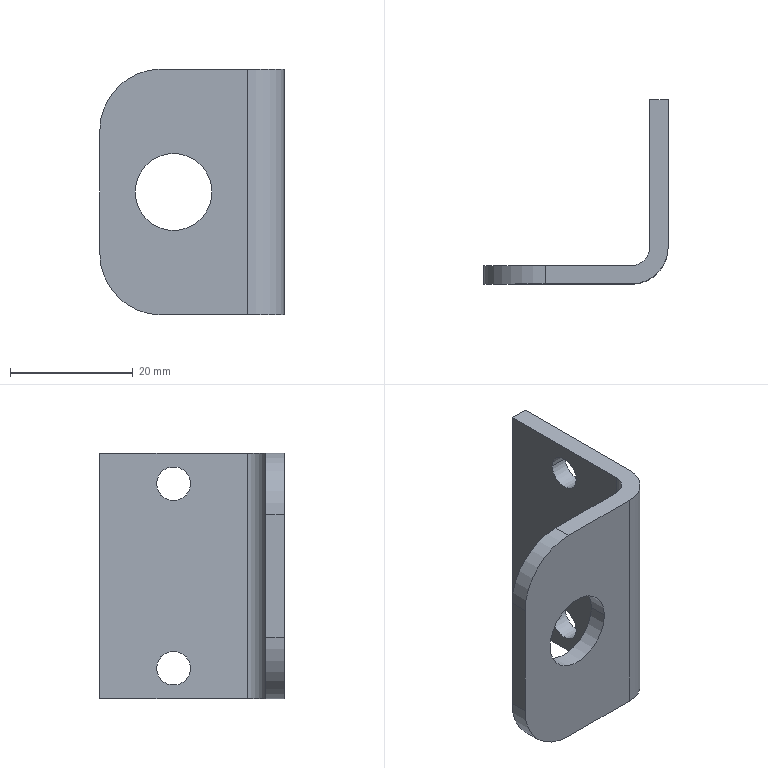Part | STEP file | X77-04002 | 1 solid | 18 faces | box 30 x 30 x 40 mm | volume 5969 mm3 | cylinder 10 | plane 8 | commonest cylinder face diameters 5.5 x4 12.5 x2 20 x2 6 x1 12 x1
STEP:
#1=CARTESIAN_POINT('',(-8.75,-30.,20.));
#2=VERTEX_POINT('',#1);
#3=CARTESIAN_POINT('',(-21.25,-30.,20.));
#4=VERTEX_POINT('',#3);
#5=CARTESIAN_POINT('',(-15.,-30.,20.));
#6=DIRECTION('',(0.,1.,0.));
#7=DIRECTION('',(-1.,0.,0.));
#8=AXIS2_PLACEMENT_3D('',#5,#6,#7);
#9=CIRCLE('',#8,6.25);
#10=EDGE_CURVE('',#2,#4,#9,.T.);
#11=ORIENTED_EDGE('',*,*,#10,.F.);
#12=CARTESIAN_POINT('',(-8.75,-27.,20.));
#13=VERTEX_POINT('',#12);
#14=CARTESIAN_POINT('',(-8.75,-30.,20.));
#15=DIRECTION('',(0.,1.,0.));
#16=VECTOR('',#15,1000.);
#17=LINE('',#14,#16);
#18=EDGE_CURVE('',#2,#13,#17,.T.);
#19=ORIENTED_EDGE('',*,*,#18,.T.);
#20=CARTESIAN_POINT('',(-21.25,-27.,20.));
#21=VERTEX_POINT('',#20);
#22=CARTESIAN_POINT('',(-15.,-27.,20.));
#23=DIRECTION('',(0.,1.,0.));
#24=DIRECTION('',(-1.,0.,0.));
#25=AXIS2_PLACEMENT_3D('',#22,#23,#24);
#26=CIRCLE('',#25,6.25);
#27=EDGE_CURVE('',#13,#21,#26,.T.);
#28=ORIENTED_EDGE('',*,*,#27,.T.);
#29=CARTESIAN_POINT('',(-21.25,-30.,20.));
#30=DIRECTION('',(0.,1.,0.));
#31=VECTOR('',#30,1000.);
#32=LINE('',#29,#31);
#33=EDGE_CURVE('',#4,#21,#32,.T.);
#34=ORIENTED_EDGE('',*,*,#33,.F.);
#35=EDGE_LOOP('',(#11,#19,#28,#34));
#36=FACE_OUTER_BOUND('',#35,.T.);
#37=CARTESIAN_POINT('',(-15.,-30.,20.));
#38=DIRECTION('',(0.,1.,0.));
#39=DIRECTION('',(-1.,0.,0.));
#40=AXIS2_PLACEMENT_3D('',#37,#38,#39);
#41=CYLINDRICAL_SURFACE('',#40,6.25);
#42=ADVANCED_FACE('',(#36),#41,.F.);
#43=CARTESIAN_POINT('',(3.,-9.25,35.));
#44=VERTEX_POINT('',#43);
#45=CARTESIAN_POINT('',(3.,-14.75,35.));
#46=VERTEX_POINT('',#45);
#47=CARTESIAN_POINT('',(3.,-12.,35.));
#48=DIRECTION('',(-1.,0.,0.));
#49=DIRECTION('',(0.,-1.,0.));
#50=AXIS2_PLACEMENT_3D('',#47,#48,#49);
#51=CIRCLE('',#50,2.75);
#52=EDGE_CURVE('',#44,#46,#51,.T.);
#53=ORIENTED_EDGE('',*,*,#52,.F.);
#54=CARTESIAN_POINT('',(0.,-9.25,35.));
#55=VERTEX_POINT('',#54);
#56=CARTESIAN_POINT('',(3.,-9.25,35.));
#57=DIRECTION('',(-1.,0.,0.));
#58=VECTOR('',#57,1000.);
#59=LINE('',#56,#58);
#60=EDGE_CURVE('',#44,#55,#59,.T.);
#61=ORIENTED_EDGE('',*,*,#60,.T.);
#62=CARTESIAN_POINT('',(0.,-14.75,35.));
#63=VERTEX_POINT('',#62);
#64=CARTESIAN_POINT('',(0.,-12.,35.));
#65=DIRECTION('',(-1.,0.,0.));
#66=DIRECTION('',(0.,-1.,0.));
#67=AXIS2_PLACEMENT_3D('',#64,#65,#66);
#68=CIRCLE('',#67,2.75);
#69=EDGE_CURVE('',#55,#63,#68,.T.);
#70=ORIENTED_EDGE('',*,*,#69,.T.);
#71=CARTESIAN_POINT('',(3.,-14.75,35.));
#72=DIRECTION('',(-1.,0.,0.));
#73=VECTOR('',#72,1000.);
#74=LINE('',#71,#73);
#75=EDGE_CURVE('',#46,#63,#74,.T.);
#76=ORIENTED_EDGE('',*,*,#75,.F.);
#77=EDGE_LOOP('',(#53,#61,#70,#76));
#78=FACE_OUTER_BOUND('',#77,.T.);
#79=CARTESIAN_POINT('',(3.,-12.,35.));
#80=DIRECTION('',(-1.,0.,0.));
#81=DIRECTION('',(0.,-1.,0.));
#82=AXIS2_PLACEMENT_3D('',#79,#80,#81);
#83=CYLINDRICAL_SURFACE('',#82,2.75);
#84=ADVANCED_FACE('',(#78),#83,.F.);
#85=CARTESIAN_POINT('',(3.,-9.25,5.));
#86=VERTEX_POINT('',#85);
#87=CARTESIAN_POINT('',(3.,-14.75,5.));
#88=VERTEX_POINT('',#87);
#89=CARTESIAN_POINT('',(3.,-12.,5.));
#90=DIRECTION('',(-1.,0.,0.));
#91=DIRECTION('',(0.,-1.,0.));
#92=AXIS2_PLACEMENT_3D('',#89,#90,#91);
#93=CIRCLE('',#92,2.75);
#94=EDGE_CURVE('',#86,#88,#93,.T.);
#95=ORIENTED_EDGE('',*,*,#94,.F.);
#96=CARTESIAN_POINT('',(0.,-9.25,5.));
#97=VERTEX_POINT('',#96);
#98=CARTESIAN_POINT('',(3.,-9.25,5.));
#99=DIRECTION('',(-1.,0.,0.));
#100=VECTOR('',#99,1000.);
#101=LINE('',#98,#100);
#102=EDGE_CURVE('',#86,#97,#101,.T.);
#103=ORIENTED_EDGE('',*,*,#102,.T.);
#104=CARTESIAN_POINT('',(0.,-14.75,5.));
#105=VERTEX_POINT('',#104);
#106=CARTESIAN_POINT('',(0.,-12.,5.));
#107=DIRECTION('',(-1.,0.,0.));
#108=DIRECTION('',(0.,-1.,0.));
#109=AXIS2_PLACEMENT_3D('',#106,#107,#108);
#110=CIRCLE('',#109,2.75);
#111=EDGE_CURVE('',#97,#105,#110,.T.);
#112=ORIENTED_EDGE('',*,*,#111,.T.);
#113=CARTESIAN_POINT('',(3.,-14.75,5.));
#114=DIRECTION('',(-1.,0.,0.));
#115=VECTOR('',#114,1000.);
#116=LINE('',#113,#115);
#117=EDGE_CURVE('',#88,#105,#116,.T.);
#118=ORIENTED_EDGE('',*,*,#117,.F.);
#119=EDGE_LOOP('',(#95,#103,#112,#118));
#120=FACE_OUTER_BOUND('',#119,.T.);
#121=CARTESIAN_POINT('',(3.,-12.,5.));
#122=DIRECTION('',(-1.,0.,0.));
#123=DIRECTION('',(0.,-1.,0.));
#124=AXIS2_PLACEMENT_3D('',#121,#122,#123);
#125=CYLINDRICAL_SURFACE('',#124,2.75);
#126=ADVANCED_FACE('',(#120),#125,.F.);
#127=CARTESIAN_POINT('',(3.,0.,0.));
#128=VERTEX_POINT('',#127);
#129=CARTESIAN_POINT('',(0.,0.,0.));
#130=VERTEX_POINT('',#129);
#131=CARTESIAN_POINT('',(3.,0.,0.));
#132=DIRECTION('',(-1.,0.,0.));
#133=VECTOR('',#132,1000.);
#134=LINE('',#131,#133);
#135=EDGE_CURVE('',#128,#130,#134,.T.);
#136=ORIENTED_EDGE('',*,*,#135,.T.);
#137=CARTESIAN_POINT('',(0.,0.,40.));
#138=VERTEX_POINT('',#137);
#139=CARTESIAN_POINT('',(0.,0.,40.));
#140=DIRECTION('',(0.,0.,-1.));
#141=VECTOR('',#140,1000.);
#142=LINE('',#139,#141);
#143=EDGE_CURVE('',#138,#130,#142,.T.);
#144=ORIENTED_EDGE('',*,*,#143,.F.);
#145=CARTESIAN_POINT('',(3.,0.,40.));
#146=VERTEX_POINT('',#145);
#147=CARTESIAN_POINT('',(3.,0.,40.));
#148=DIRECTION('',(-1.,0.,0.));
#149=VECTOR('',#148,1000.);
#150=LINE('',#147,#149);
#151=EDGE_CURVE('',#146,#138,#150,.T.);
#152=ORIENTED_EDGE('',*,*,#151,.F.);
#153=CARTESIAN_POINT('',(3.,0.,40.));
#154=DIRECTION('',(0.,0.,-1.));
#155=VECTOR('',#154,1000.);
#156=LINE('',#153,#155);
#157=EDGE_CURVE('',#146,#128,#156,.T.);
#158=ORIENTED_EDGE('',*,*,#157,.T.);
#159=EDGE_LOOP('',(#136,#144,#152,#158));
#160=FACE_OUTER_BOUND('',#159,.T.);
#161=CARTESIAN_POINT('',(3.,0.,40.));
#162=DIRECTION('',(0.,-1.,0.));
#163=DIRECTION('',(1.,0.,0.));
#164=AXIS2_PLACEMENT_3D('',#161,#162,#163);
#165=PLANE('',#164);
#166=ADVANCED_FACE('',(#160),#165,.F.);
#167=CARTESIAN_POINT('',(0.,-12.,35.));
#168=DIRECTION('',(-1.,0.,0.));
#169=DIRECTION('',(0.,-1.,0.));
#170=AXIS2_PLACEMENT_3D('',#167,#168,#169);
#171=CIRCLE('',#170,2.75);
#172=EDGE_CURVE('',#63,#55,#171,.T.);
#173=ORIENTED_EDGE('',*,*,#172,.F.);
#174=ORIENTED_EDGE('',*,*,#69,.F.);
#175=EDGE_LOOP('',(#173,#174));
#176=FACE_BOUND('',#175,.T.);
#177=CARTESIAN_POINT('',(0.,-12.,5.));
#178=DIRECTION('',(-1.,0.,0.));
#179=DIRECTION('',(0.,-1.,0.));
#180=AXIS2_PLACEMENT_3D('',#177,#178,#179);
#181=CIRCLE('',#180,2.75);
#182=EDGE_CURVE('',#105,#97,#181,.T.);
#183=ORIENTED_EDGE('',*,*,#182,.F.);
#184=ORIENTED_EDGE('',*,*,#111,.F.);
#185=EDGE_LOOP('',(#183,#184));
#186=FACE_BOUND('',#185,.T.);
#187=CARTESIAN_POINT('',(0.,-24.,0.));
#188=VERTEX_POINT('',#187);
#189=CARTESIAN_POINT('',(0.,0.,0.));
#190=DIRECTION('',(0.,-1.,0.));
#191=VECTOR('',#190,1000.);
#192=LINE('',#189,#191);
#193=EDGE_CURVE('',#130,#188,#192,.T.);
#194=ORIENTED_EDGE('',*,*,#193,.T.);
#195=CARTESIAN_POINT('',(0.,-24.,40.));
#196=VERTEX_POINT('',#195);
#197=CARTESIAN_POINT('',(0.,-24.,40.));
#198=DIRECTION('',(0.,0.,-1.));
#199=VECTOR('',#198,1000.);
#200=LINE('',#197,#199);
#201=EDGE_CURVE('',#196,#188,#200,.T.);
#202=ORIENTED_EDGE('',*,*,#201,.F.);
#203=CARTESIAN_POINT('',(0.,0.,40.));
#204=DIRECTION('',(0.,-1.,0.));
#205=VECTOR('',#204,1000.);
#206=LINE('',#203,#205);
#207=EDGE_CURVE('',#138,#196,#206,.T.);
#208=ORIENTED_EDGE('',*,*,#207,.F.);
#209=ORIENTED_EDGE('',*,*,#143,.T.);
#210=EDGE_LOOP('',(#194,#202,#208,#209));
#211=FACE_OUTER_BOUND('',#210,.T.);
#212=CARTESIAN_POINT('',(0.,0.,40.));
#213=DIRECTION('',(1.,0.,0.));
#214=DIRECTION('',(0.,1.,0.));
#215=AXIS2_PLACEMENT_3D('',#212,#213,#214);
#216=PLANE('',#215);
#217=ADVANCED_FACE('',(#176,#186,#211),#216,.F.);
#218=CARTESIAN_POINT('',(-3.,-27.,0.));
#219=VERTEX_POINT('',#218);
#220=CARTESIAN_POINT('',(-3.,-24.,0.));
#221=DIRECTION('',(0.,0.,-1.));
#222=DIRECTION('',(1.,0.,0.));
#223=AXIS2_PLACEMENT_3D('',#220,#221,#222);
#224=CIRCLE('',#223,3.);
#225=EDGE_CURVE('',#188,#219,#224,.T.);
#226=ORIENTED_EDGE('',*,*,#225,.T.);
#227=CARTESIAN_POINT('',(-3.,-27.,40.));
#228=VERTEX_POINT('',#227);
#229=CARTESIAN_POINT('',(-3.,-27.,40.));
#230=DIRECTION('',(0.,0.,-1.));
#231=VECTOR('',#230,1000.);
#232=LINE('',#229,#231);
#233=EDGE_CURVE('',#228,#219,#232,.T.);
#234=ORIENTED_EDGE('',*,*,#233,.F.);
#235=CARTESIAN_POINT('',(-3.,-24.,40.));
#236=DIRECTION('',(0.,0.,-1.));
#237=DIRECTION('',(1.,0.,0.));
#238=AXIS2_PLACEMENT_3D('',#235,#236,#237);
#239=CIRCLE('',#238,3.);
#240=EDGE_CURVE('',#196,#228,#239,.T.);
#241=ORIENTED_EDGE('',*,*,#240,.F.);
#242=ORIENTED_EDGE('',*,*,#201,.T.);
#243=EDGE_LOOP('',(#226,#234,#241,#242));
#244=FACE_OUTER_BOUND('',#243,.T.);
#245=CARTESIAN_POINT('',(-3.,-24.,40.));
#246=DIRECTION('',(0.,0.,-1.));
#247=DIRECTION('',(-1.,0.,0.));
#248=AXIS2_PLACEMENT_3D('',#245,#246,#247);
#249=CYLINDRICAL_SURFACE('',#248,3.);
#250=ADVANCED_FACE('',(#244),#249,.F.);
#251=CARTESIAN_POINT('',(-15.,-27.,20.));
#252=DIRECTION('',(0.,1.,0.));
#253=DIRECTION('',(-1.,0.,0.));
#254=AXIS2_PLACEMENT_3D('',#251,#252,#253);
#255=CIRCLE('',#254,6.25);
#256=EDGE_CURVE('',#21,#13,#255,.T.);
#257=ORIENTED_EDGE('',*,*,#256,.F.);
#258=ORIENTED_EDGE('',*,*,#27,.F.);
#259=EDGE_LOOP('',(#257,#258));
#260=FACE_BOUND('',#259,.T.);
#261=CARTESIAN_POINT('',(-27.,-27.,30.));
#262=VERTEX_POINT('',#261);
#263=CARTESIAN_POINT('',(-27.,-27.,10.));
#264=VERTEX_POINT('',#263);
#265=CARTESIAN_POINT('',(-27.,-27.,40.));
#266=DIRECTION('',(0.,0.,-1.));
#267=VECTOR('',#266,1000.);
#268=LINE('',#265,#267);
#269=EDGE_CURVE('',#262,#264,#268,.T.);
#270=ORIENTED_EDGE('',*,*,#269,.F.);
#271=CARTESIAN_POINT('',(-17.,-27.,40.));
#272=VERTEX_POINT('',#271);
#273=CARTESIAN_POINT('',(-17.,-27.,30.));
#274=DIRECTION('',(0.,1.,0.));
#275=DIRECTION('',(1.,0.,0.));
#276=AXIS2_PLACEMENT_3D('',#273,#274,#275);
#277=CIRCLE('',#276,10.);
#278=EDGE_CURVE('',#262,#272,#277,.T.);
#279=ORIENTED_EDGE('',*,*,#278,.T.);
#280=CARTESIAN_POINT('',(-3.,-27.,40.));
#281=DIRECTION('',(-1.,0.,0.));
#282=VECTOR('',#281,1000.);
#283=LINE('',#280,#282);
#284=EDGE_CURVE('',#228,#272,#283,.T.);
#285=ORIENTED_EDGE('',*,*,#284,.F.);
#286=ORIENTED_EDGE('',*,*,#233,.T.);
#287=CARTESIAN_POINT('',(-17.,-27.,0.));
#288=VERTEX_POINT('',#287);
#289=CARTESIAN_POINT('',(-3.,-27.,0.));
#290=DIRECTION('',(-1.,0.,0.));
#291=VECTOR('',#290,1000.);
#292=LINE('',#289,#291);
#293=EDGE_CURVE('',#219,#288,#292,.T.);
#294=ORIENTED_EDGE('',*,*,#293,.T.);
#295=CARTESIAN_POINT('',(-17.,-27.,10.));
#296=DIRECTION('',(0.,1.,0.));
#297=DIRECTION('',(1.,0.,0.));
#298=AXIS2_PLACEMENT_3D('',#295,#296,#297);
#299=CIRCLE('',#298,10.);
#300=EDGE_CURVE('',#288,#264,#299,.T.);
#301=ORIENTED_EDGE('',*,*,#300,.T.);
#302=EDGE_LOOP('',(#270,#279,#285,#286,#294,#301));
#303=FACE_OUTER_BOUND('',#302,.T.);
#304=CARTESIAN_POINT('',(-3.,-27.,40.));
#305=DIRECTION('',(0.,-1.,0.));
#306=DIRECTION('',(1.,0.,0.));
#307=AXIS2_PLACEMENT_3D('',#304,#305,#306);
#308=PLANE('',#307);
#309=ADVANCED_FACE('',(#260,#303),#308,.F.);
#310=CARTESIAN_POINT('',(-27.,-30.,30.));
#311=VERTEX_POINT('',#310);
#312=CARTESIAN_POINT('',(-27.,-30.,10.));
#313=VERTEX_POINT('',#312);
#314=CARTESIAN_POINT('',(-27.,-30.,40.));
#315=DIRECTION('',(0.,0.,-1.));
#316=VECTOR('',#315,1000.);
#317=LINE('',#314,#316);
#318=EDGE_CURVE('',#311,#313,#317,.T.);
#319=ORIENTED_EDGE('',*,*,#318,.F.);
#320=CARTESIAN_POINT('',(-27.,-27.,30.));
#321=DIRECTION('',(0.,1.,0.));
#322=VECTOR('',#321,1000.);
#323=LINE('',#320,#322);
#324=EDGE_CURVE('',#311,#262,#323,.T.);
#325=ORIENTED_EDGE('',*,*,#324,.T.);
#326=ORIENTED_EDGE('',*,*,#269,.T.);
#327=CARTESIAN_POINT('',(-27.,-27.,10.));
#328=DIRECTION('',(0.,-1.,0.));
#329=VECTOR('',#328,1000.);
#330=LINE('',#327,#329);
#331=EDGE_CURVE('',#264,#313,#330,.T.);
#332=ORIENTED_EDGE('',*,*,#331,.T.);
#333=EDGE_LOOP('',(#319,#325,#326,#332));
#334=FACE_OUTER_BOUND('',#333,.T.);
#335=CARTESIAN_POINT('',(-27.,-27.,40.));
#336=DIRECTION('',(1.,0.,0.));
#337=DIRECTION('',(0.,1.,0.));
#338=AXIS2_PLACEMENT_3D('',#335,#336,#337);
#339=PLANE('',#338);
#340=ADVANCED_FACE('',(#334),#339,.F.);
#341=CARTESIAN_POINT('',(-15.,-30.,20.));
#342=DIRECTION('',(0.,1.,0.));
#343=DIRECTION('',(-1.,0.,0.));
#344=AXIS2_PLACEMENT_3D('',#341,#342,#343);
#345=CIRCLE('',#344,6.25);
#346=EDGE_CURVE('',#4,#2,#345,.T.);
#347=ORIENTED_EDGE('',*,*,#346,.T.);
#348=ORIENTED_EDGE('',*,*,#10,.T.);
#349=EDGE_LOOP('',(#347,#348));
#350=FACE_BOUND('',#349,.T.);
#351=CARTESIAN_POINT('',(-17.,-30.,40.));
#352=VERTEX_POINT('',#351);
#353=CARTESIAN_POINT('',(-3.,-30.,40.));
#354=VERTEX_POINT('',#353);
#355=CARTESIAN_POINT('',(-27.,-30.,40.));
#356=DIRECTION('',(1.,0.,0.));
#357=VECTOR('',#356,1000.);
#358=LINE('',#355,#357);
#359=EDGE_CURVE('',#352,#354,#358,.T.);
#360=ORIENTED_EDGE('',*,*,#359,.F.);
#361=CARTESIAN_POINT('',(-17.,-30.,30.));
#362=DIRECTION('',(0.,-1.,0.));
#363=DIRECTION('',(0.,0.,1.));
#364=AXIS2_PLACEMENT_3D('',#361,#362,#363);
#365=CIRCLE('',#364,10.);
#366=EDGE_CURVE('',#352,#311,#365,.T.);
#367=ORIENTED_EDGE('',*,*,#366,.T.);
#368=ORIENTED_EDGE('',*,*,#318,.T.);
#369=CARTESIAN_POINT('',(-17.,-30.,0.));
#370=VERTEX_POINT('',#369);
#371=CARTESIAN_POINT('',(-17.,-30.,10.));
#372=DIRECTION('',(0.,-1.,0.));
#373=DIRECTION('',(0.,0.,1.));
#374=AXIS2_PLACEMENT_3D('',#371,#372,#373);
#375=CIRCLE('',#374,10.);
#376=EDGE_CURVE('',#313,#370,#375,.T.);
#377=ORIENTED_EDGE('',*,*,#376,.T.);
#378=CARTESIAN_POINT('',(-3.,-30.,0.));
#379=VERTEX_POINT('',#378);
#380=CARTESIAN_POINT('',(-27.,-30.,0.));
#381=DIRECTION('',(1.,0.,0.));
#382=VECTOR('',#381,1000.);
#383=LINE('',#380,#382);
#384=EDGE_CURVE('',#370,#379,#383,.T.);
#385=ORIENTED_EDGE('',*,*,#384,.T.);
#386=CARTESIAN_POINT('',(-3.,-30.,40.));
#387=DIRECTION('',(0.,0.,-1.));
#388=VECTOR('',#387,1000.);
#389=LINE('',#386,#388);
#390=EDGE_CURVE('',#354,#379,#389,.T.);
#391=ORIENTED_EDGE('',*,*,#390,.F.);
#392=EDGE_LOOP('',(#360,#367,#368,#377,#385,#391));
#393=FACE_OUTER_BOUND('',#392,.T.);
#394=CARTESIAN_POINT('',(-27.,-30.,40.));
#395=DIRECTION('',(0.,1.,0.));
#396=DIRECTION('',(0.,0.,1.));
#397=AXIS2_PLACEMENT_3D('',#394,#395,#396);
#398=PLANE('',#397);
#399=ADVANCED_FACE('',(#350,#393),#398,.F.);
#400=CARTESIAN_POINT('',(3.,-24.,0.));
#401=VERTEX_POINT('',#400);
#402=CARTESIAN_POINT('',(-3.,-24.,0.));
#403=DIRECTION('',(0.,0.,1.));
#404=DIRECTION('',(1.,0.,0.));
#405=AXIS2_PLACEMENT_3D('',#402,#403,#404);
#406=CIRCLE('',#405,6.);
#407=EDGE_CURVE('',#379,#401,#406,.T.);
#408=ORIENTED_EDGE('',*,*,#407,.T.);
#409=CARTESIAN_POINT('',(3.,-24.,40.));
#410=VERTEX_POINT('',#409);
#411=CARTESIAN_POINT('',(3.,-24.,40.));
#412=DIRECTION('',(0.,0.,-1.));
#413=VECTOR('',#412,1000.);
#414=LINE('',#411,#413);
#415=EDGE_CURVE('',#410,#401,#414,.T.);
#416=ORIENTED_EDGE('',*,*,#415,.F.);
#417=CARTESIAN_POINT('',(-3.,-24.,40.));
#418=DIRECTION('',(0.,0.,1.));
#419=DIRECTION('',(1.,0.,0.));
#420=AXIS2_PLACEMENT_3D('',#417,#418,#419);
#421=CIRCLE('',#420,6.);
#422=EDGE_CURVE('',#354,#410,#421,.T.);
#423=ORIENTED_EDGE('',*,*,#422,.F.);
#424=ORIENTED_EDGE('',*,*,#390,.T.);
#425=EDGE_LOOP('',(#408,#416,#423,#424));
#426=FACE_OUTER_BOUND('',#425,.T.);
#427=CARTESIAN_POINT('',(-3.,-24.,40.));
#428=DIRECTION('',(0.,0.,-1.));
#429=DIRECTION('',(-1.,0.,0.));
#430=AXIS2_PLACEMENT_3D('',#427,#428,#429);
#431=CYLINDRICAL_SURFACE('',#430,6.);
#432=ADVANCED_FACE('',(#426),#431,.T.);
#433=CARTESIAN_POINT('',(3.,-12.,35.));
#434=DIRECTION('',(-1.,0.,0.));
#435=DIRECTION('',(0.,-1.,0.));
#436=AXIS2_PLACEMENT_3D('',#433,#434,#435);
#437=CIRCLE('',#436,2.75);
#438=EDGE_CURVE('',#46,#44,#437,.T.);
#439=ORIENTED_EDGE('',*,*,#438,.T.);
#440=ORIENTED_EDGE('',*,*,#52,.T.);
#441=EDGE_LOOP('',(#439,#440));
#442=FACE_BOUND('',#441,.T.);
#443=CARTESIAN_POINT('',(3.,-12.,5.));
#444=DIRECTION('',(-1.,0.,0.));
#445=DIRECTION('',(0.,-1.,0.));
#446=AXIS2_PLACEMENT_3D('',#443,#444,#445);
#447=CIRCLE('',#446,2.75);
#448=EDGE_CURVE('',#88,#86,#447,.T.);
#449=ORIENTED_EDGE('',*,*,#448,.T.);
#450=ORIENTED_EDGE('',*,*,#94,.T.);
#451=EDGE_LOOP('',(#449,#450));
#452=FACE_BOUND('',#451,.T.);
#453=CARTESIAN_POINT('',(3.,-24.,0.));
#454=DIRECTION('',(0.,1.,0.));
#455=VECTOR('',#454,1000.);
#456=LINE('',#453,#455);
#457=EDGE_CURVE('',#401,#128,#456,.T.);
#458=ORIENTED_EDGE('',*,*,#457,.T.);
#459=ORIENTED_EDGE('',*,*,#157,.F.);
#460=CARTESIAN_POINT('',(3.,-24.,40.));
#461=DIRECTION('',(0.,1.,0.));
#462=VECTOR('',#461,1000.);
#463=LINE('',#460,#462);
#464=EDGE_CURVE('',#410,#146,#463,.T.);
#465=ORIENTED_EDGE('',*,*,#464,.F.);
#466=ORIENTED_EDGE('',*,*,#415,.T.);
#467=EDGE_LOOP('',(#458,#459,#465,#466));
#468=FACE_OUTER_BOUND('',#467,.T.);
#469=CARTESIAN_POINT('',(3.,-24.,40.));
#470=DIRECTION('',(-1.,0.,0.));
#471=DIRECTION('',(0.,0.,1.));
#472=AXIS2_PLACEMENT_3D('',#469,#470,#471);
#473=PLANE('',#472);
#474=ADVANCED_FACE('',(#442,#452,#468),#473,.F.);
#475=ORIENTED_EDGE('',*,*,#284,.T.);
#476=CARTESIAN_POINT('',(-17.,-30.,40.));
#477=DIRECTION('',(0.,-1.,0.));
#478=VECTOR('',#477,1000.);
#479=LINE('',#476,#478);
#480=EDGE_CURVE('',#272,#352,#479,.T.);
#481=ORIENTED_EDGE('',*,*,#480,.T.);
#482=ORIENTED_EDGE('',*,*,#359,.T.);
#483=ORIENTED_EDGE('',*,*,#422,.T.);
#484=ORIENTED_EDGE('',*,*,#464,.T.);
#485=ORIENTED_EDGE('',*,*,#151,.T.);
#486=ORIENTED_EDGE('',*,*,#207,.T.);
#487=ORIENTED_EDGE('',*,*,#240,.T.);
#488=EDGE_LOOP('',(#475,#481,#482,#483,#484,#485,#486,#487));
#489=FACE_OUTER_BOUND('',#488,.T.);
#490=CARTESIAN_POINT('',(-3.,-24.,40.));
#491=DIRECTION('',(0.,0.,1.));
#492=DIRECTION('',(1.,0.,0.));
#493=AXIS2_PLACEMENT_3D('',#490,#491,#492);
#494=PLANE('',#493);
#495=ADVANCED_FACE('',(#489),#494,.T.);
#496=ORIENTED_EDGE('',*,*,#384,.F.);
#497=CARTESIAN_POINT('',(-17.,-24.,0.));
#498=DIRECTION('',(0.,1.,0.));
#499=VECTOR('',#498,1000.);
#500=LINE('',#497,#499);
#501=EDGE_CURVE('',#370,#288,#500,.T.);
#502=ORIENTED_EDGE('',*,*,#501,.T.);
#503=ORIENTED_EDGE('',*,*,#293,.F.);
#504=ORIENTED_EDGE('',*,*,#225,.F.);
#505=ORIENTED_EDGE('',*,*,#193,.F.);
#506=ORIENTED_EDGE('',*,*,#135,.F.);
#507=ORIENTED_EDGE('',*,*,#457,.F.);
#508=ORIENTED_EDGE('',*,*,#407,.F.);
#509=EDGE_LOOP('',(#496,#502,#503,#504,#505,#506,#507,#508));
#510=FACE_OUTER_BOUND('',#509,.T.);
#511=CARTESIAN_POINT('',(-3.,-24.,0.));
#512=DIRECTION('',(0.,0.,1.));
#513=DIRECTION('',(1.,0.,0.));
#514=AXIS2_PLACEMENT_3D('',#511,#512,#513);
#515=PLANE('',#514);
#516=ADVANCED_FACE('',(#510),#515,.F.);
#517=ORIENTED_EDGE('',*,*,#102,.F.);
#518=ORIENTED_EDGE('',*,*,#448,.F.);
#519=ORIENTED_EDGE('',*,*,#117,.T.);
#520=ORIENTED_EDGE('',*,*,#182,.T.);
#521=EDGE_LOOP('',(#517,#518,#519,#520));
#522=FACE_OUTER_BOUND('',#521,.T.);
#523=CARTESIAN_POINT('',(3.,-12.,5.));
#524=DIRECTION('',(-1.,0.,0.));
#525=DIRECTION('',(0.,-1.,0.));
#526=AXIS2_PLACEMENT_3D('',#523,#524,#525);
#527=CYLINDRICAL_SURFACE('',#526,2.75);
#528=ADVANCED_FACE('',(#522),#527,.F.);
#529=ORIENTED_EDGE('',*,*,#60,.F.);
#530=ORIENTED_EDGE('',*,*,#438,.F.);
#531=ORIENTED_EDGE('',*,*,#75,.T.);
#532=ORIENTED_EDGE('',*,*,#172,.T.);
#533=EDGE_LOOP('',(#529,#530,#531,#532));
#534=FACE_OUTER_BOUND('',#533,.T.);
#535=CARTESIAN_POINT('',(3.,-12.,35.));
#536=DIRECTION('',(-1.,0.,0.));
#537=DIRECTION('',(0.,-1.,0.));
#538=AXIS2_PLACEMENT_3D('',#535,#536,#537);
#539=CYLINDRICAL_SURFACE('',#538,2.75);
#540=ADVANCED_FACE('',(#534),#539,.F.);
#541=ORIENTED_EDGE('',*,*,#18,.F.);
#542=ORIENTED_EDGE('',*,*,#346,.F.);
#543=ORIENTED_EDGE('',*,*,#33,.T.);
#544=ORIENTED_EDGE('',*,*,#256,.T.);
#545=EDGE_LOOP('',(#541,#542,#543,#544));
#546=FACE_OUTER_BOUND('',#545,.T.);
#547=CARTESIAN_POINT('',(-15.,-30.,20.));
#548=DIRECTION('',(0.,1.,0.));
#549=DIRECTION('',(-1.,0.,0.));
#550=AXIS2_PLACEMENT_3D('',#547,#548,#549);
#551=CYLINDRICAL_SURFACE('',#550,6.25);
#552=ADVANCED_FACE('',(#546),#551,.F.);
#553=ORIENTED_EDGE('',*,*,#278,.F.);
#554=ORIENTED_EDGE('',*,*,#324,.F.);
#555=ORIENTED_EDGE('',*,*,#366,.F.);
#556=ORIENTED_EDGE('',*,*,#480,.F.);
#557=EDGE_LOOP('',(#553,#554,#555,#556));
#558=FACE_OUTER_BOUND('',#557,.T.);
#559=CARTESIAN_POINT('',(-17.,-24.,30.));
#560=DIRECTION('',(0.,1.,0.));
#561=DIRECTION('',(-1.,0.,0.));
#562=AXIS2_PLACEMENT_3D('',#559,#560,#561);
#563=CYLINDRICAL_SURFACE('',#562,10.);
#564=ADVANCED_FACE('',(#558),#563,.T.);
#565=ORIENTED_EDGE('',*,*,#300,.F.);
#566=ORIENTED_EDGE('',*,*,#501,.F.);
#567=ORIENTED_EDGE('',*,*,#376,.F.);
#568=ORIENTED_EDGE('',*,*,#331,.F.);
#569=EDGE_LOOP('',(#565,#566,#567,#568));
#570=FACE_OUTER_BOUND('',#569,.T.);
#571=CARTESIAN_POINT('',(-17.,-27.,10.));
#572=DIRECTION('',(0.,-1.,0.));
#573=DIRECTION('',(1.,0.,0.));
#574=AXIS2_PLACEMENT_3D('',#571,#572,#573);
#575=CYLINDRICAL_SURFACE('',#574,10.);
#576=ADVANCED_FACE('',(#570),#575,.T.);
#577=CLOSED_SHELL('',(#42,#84,#126,#166,#217,#250,#309,#340,#399,#432,#474,#495,#516,#528,#540,#552,#564,#576));
#578=MANIFOLD_SOLID_BREP('',#577);
#579=CARTESIAN_POINT('',(0.,0.,0.));
#580=DIRECTION('',(0.,0.,1.));
#581=DIRECTION('',(1.,0.,0.));
#582=AXIS2_PLACEMENT_3D('',#579,#580,#581);
#583=(LENGTH_UNIT()NAMED_UNIT(*)SI_UNIT(.MILLI.,.METRE.));
#584=UNCERTAINTY_MEASURE_WITH_UNIT(LENGTH_MEASURE(0.00001),#583,'','');
#585=(NAMED_UNIT(*)PLANE_ANGLE_UNIT()SI_UNIT($,.RADIAN.));
#586=(NAMED_UNIT(*)SI_UNIT($,.STERADIAN.)SOLID_ANGLE_UNIT());
#587=(GEOMETRIC_REPRESENTATION_CONTEXT(3)GLOBAL_UNCERTAINTY_ASSIGNED_CONTEXT((#584))GLOBAL_UNIT_ASSIGNED_CONTEXT((#583,#585,#586))REPRESENTATION_CONTEXT('',''));
#588=ADVANCED_BREP_SHAPE_REPRESENTATION('',(#578,#582),#587);